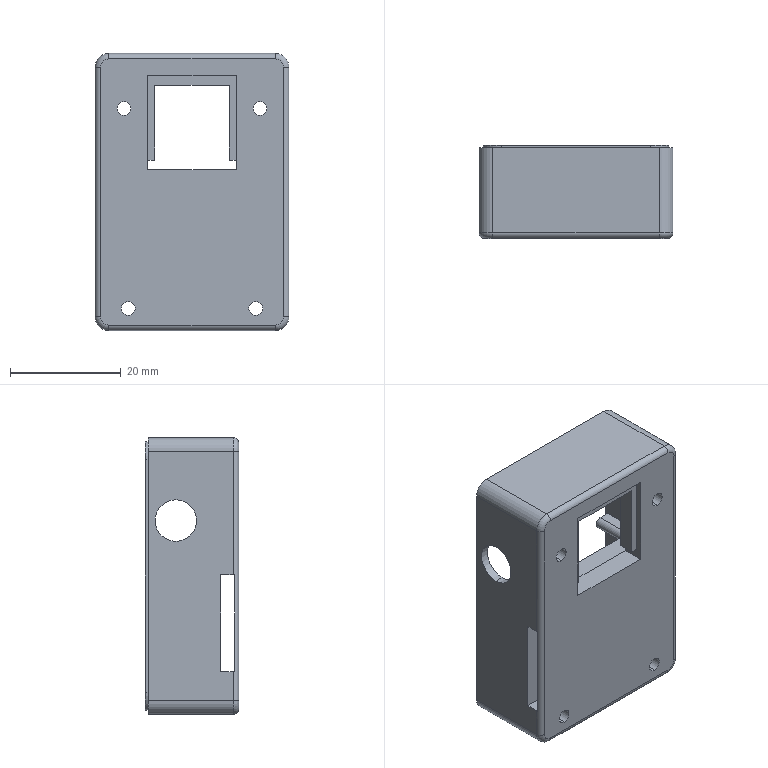Part | SolidWorks | features ICE 14, Fillet 3, MoveFace 2, Extrusion 1, HoleWzd 1, Scale 1 | 1 solid | 165 faces | box 35 x 16.85 x 50 mm | volume 10296 mm3 | cylinder 82 | plane 63 | cone 16 | torus 4 | commonest cylinder face diameters 2 x22 0.75 x20 0.8 x8 2.5 x8 5 x8 6.5 x4